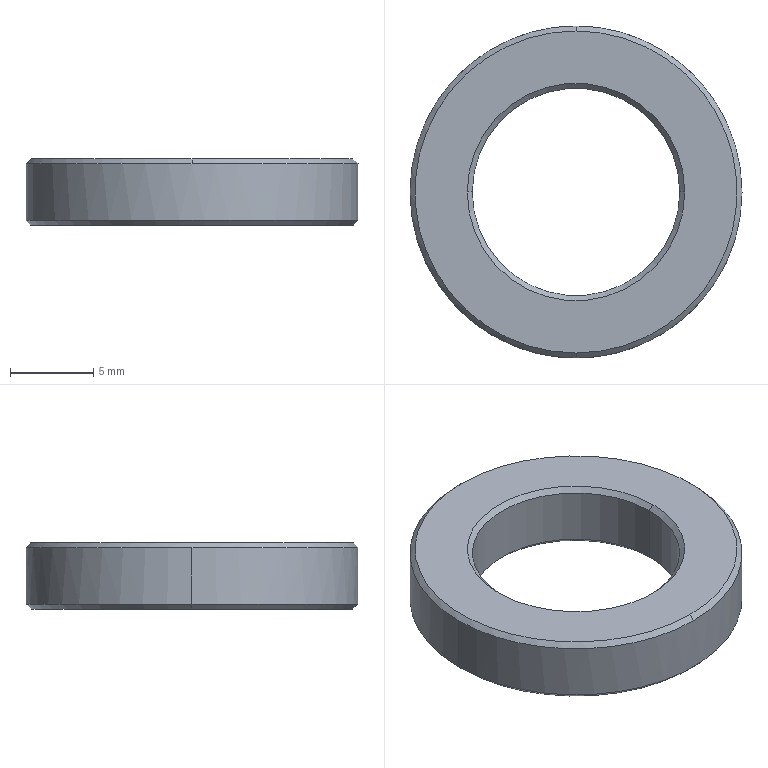Part | STEP file | Bearing locating ring | 1 solid | 14 faces | box 20 x 20 x 4 mm | volume 756.574 mm3 | cone 8 | cylinder 4 | plane 2 | commonest cylinder face diameters 12.5 x2 20 x2
STEP:
#1=CARTESIAN_POINT('',(0.,0.,0.));
#2=DIRECTION('',(0.,0.,1.));
#3=DIRECTION('',(1.,0.,0.));
#4=AXIS2_PLACEMENT_3D('',#1,#2,#3);
#5=CARTESIAN_POINT('',(10.,0.,0.3));
#6=VERTEX_POINT('',#5);
#7=CARTESIAN_POINT('',(-10.,0.,0.3));
#8=VERTEX_POINT('',#7);
#9=CARTESIAN_POINT('',(0.,0.,0.3));
#10=DIRECTION('',(0.,0.,1.));
#11=DIRECTION('',(1.,0.,0.));
#12=AXIS2_PLACEMENT_3D('',#9,#10,#11);
#13=CIRCLE('',#12,10.);
#14=CARTESIAN_POINT('',(0.,0.,0.));
#15=DIRECTION('',(0.,0.,1.));
#16=DIRECTION('',(1.,0.,0.));
#17=AXIS2_PLACEMENT_3D('',#14,#15,#16);
#18=CYLINDRICAL_SURFACE('',#17,10.);
#19=CARTESIAN_POINT('',(0.,0.3));
#20=DIRECTION('',(1.,0.));
#21=VECTOR('',#20,1.);
#22=LINE('',#19,#21);
#23=(GEOMETRIC_REPRESENTATION_CONTEXT(2)PARAMETRIC_REPRESENTATION_CONTEXT()REPRESENTATION_CONTEXT('',''));
#24=DEFINITIONAL_REPRESENTATION('',(#22),#23);
#25=PCURVE('',#18,#24);
#26=CARTESIAN_POINT('',(0.,0.,0.3));
#27=DIRECTION('',(0.,0.,1.));
#28=DIRECTION('',(1.,0.,0.));
#29=AXIS2_PLACEMENT_3D('',#26,#27,#28);
#30=CONICAL_SURFACE('',#29,10.,0.7854);
#31=CARTESIAN_POINT('',(0.,0.));
#32=DIRECTION('',(1.,0.));
#33=VECTOR('',#32,1.);
#34=LINE('',#31,#33);
#35=(GEOMETRIC_REPRESENTATION_CONTEXT(2)PARAMETRIC_REPRESENTATION_CONTEXT()REPRESENTATION_CONTEXT('',''));
#36=DEFINITIONAL_REPRESENTATION('',(#34),#35);
#37=PCURVE('',#30,#36);
#38=SURFACE_CURVE('',#13,(#25,#37),.PCURVE_S1.);
#39=EDGE_CURVE('',#6,#8,#38,.T.);
#40=ORIENTED_EDGE('',*,*,#39,.T.);
#41=CARTESIAN_POINT('',(-10.,0.,3.7));
#42=VERTEX_POINT('',#41);
#43=CARTESIAN_POINT('',(-10.,0.,0.));
#44=DIRECTION('',(0.,0.,1.));
#45=VECTOR('',#44,1.);
#46=LINE('',#43,#45);
#47=CARTESIAN_POINT('',(3.142,0.));
#48=DIRECTION('',(0.,1.));
#49=VECTOR('',#48,1.);
#50=LINE('',#47,#49);
#51=(GEOMETRIC_REPRESENTATION_CONTEXT(2)PARAMETRIC_REPRESENTATION_CONTEXT()REPRESENTATION_CONTEXT('',''));
#52=DEFINITIONAL_REPRESENTATION('',(#50),#51);
#53=PCURVE('',#18,#52);
#54=CARTESIAN_POINT('',(0.,0.,0.));
#55=DIRECTION('',(0.,0.,1.));
#56=DIRECTION('',(1.,0.,0.));
#57=AXIS2_PLACEMENT_3D('',#54,#55,#56);
#58=CYLINDRICAL_SURFACE('',#57,10.);
#59=CARTESIAN_POINT('',(3.142,0.));
#60=DIRECTION('',(0.,1.));
#61=VECTOR('',#60,1.);
#62=LINE('',#59,#61);
#63=(GEOMETRIC_REPRESENTATION_CONTEXT(2)PARAMETRIC_REPRESENTATION_CONTEXT()REPRESENTATION_CONTEXT('',''));
#64=DEFINITIONAL_REPRESENTATION('',(#62),#63);
#65=PCURVE('',#58,#64);
#66=SURFACE_CURVE('',#46,(#53,#65),.PCURVE_S1.);
#67=EDGE_CURVE('',#8,#42,#66,.T.);
#68=ORIENTED_EDGE('',*,*,#67,.T.);
#69=CARTESIAN_POINT('',(0.,10.,3.7));
#70=VERTEX_POINT('',#69);
#71=CARTESIAN_POINT('',(0.,0.,3.7));
#72=DIRECTION('',(0.,0.,-1.));
#73=DIRECTION('',(1.,0.,0.));
#74=AXIS2_PLACEMENT_3D('',#71,#72,#73);
#75=CIRCLE('',#74,10.);
#76=CARTESIAN_POINT('',(6.283,3.7));
#77=DIRECTION('',(-1.,0.));
#78=VECTOR('',#77,1.);
#79=LINE('',#76,#78);
#80=(GEOMETRIC_REPRESENTATION_CONTEXT(2)PARAMETRIC_REPRESENTATION_CONTEXT()REPRESENTATION_CONTEXT('',''));
#81=DEFINITIONAL_REPRESENTATION('',(#79),#80);
#82=PCURVE('',#18,#81);
#83=CARTESIAN_POINT('',(0.,0.,3.7));
#84=DIRECTION('',(0.,0.,-1.));
#85=DIRECTION('',(0.,1.,0.));
#86=AXIS2_PLACEMENT_3D('',#83,#84,#85);
#87=CONICAL_SURFACE('',#86,10.,0.7854);
#88=CARTESIAN_POINT('',(1.571,0.));
#89=DIRECTION('',(1.,0.));
#90=VECTOR('',#89,1.);
#91=LINE('',#88,#90);
#92=(GEOMETRIC_REPRESENTATION_CONTEXT(2)PARAMETRIC_REPRESENTATION_CONTEXT()REPRESENTATION_CONTEXT('',''));
#93=DEFINITIONAL_REPRESENTATION('',(#91),#92);
#94=PCURVE('',#87,#93);
#95=SURFACE_CURVE('',#75,(#82,#94),.PCURVE_S1.);
#96=EDGE_CURVE('',#42,#70,#95,.T.);
#97=ORIENTED_EDGE('',*,*,#96,.T.);
#98=CARTESIAN_POINT('',(10.,0.,3.7));
#99=VERTEX_POINT('',#98);
#100=CARTESIAN_POINT('',(0.,0.,3.7));
#101=DIRECTION('',(0.,0.,-1.));
#102=DIRECTION('',(1.,0.,0.));
#103=AXIS2_PLACEMENT_3D('',#100,#101,#102);
#104=CIRCLE('',#103,10.);
#105=CARTESIAN_POINT('',(6.283,3.7));
#106=DIRECTION('',(-1.,0.));
#107=VECTOR('',#106,1.);
#108=LINE('',#105,#107);
#109=(GEOMETRIC_REPRESENTATION_CONTEXT(2)PARAMETRIC_REPRESENTATION_CONTEXT()REPRESENTATION_CONTEXT('',''));
#110=DEFINITIONAL_REPRESENTATION('',(#108),#109);
#111=PCURVE('',#18,#110);
#112=CARTESIAN_POINT('',(0.,0.,3.7));
#113=DIRECTION('',(0.,0.,-1.));
#114=DIRECTION('',(0.,1.,0.));
#115=AXIS2_PLACEMENT_3D('',#112,#113,#114);
#116=CONICAL_SURFACE('',#115,10.,0.7854);
#117=CARTESIAN_POINT('',(-4.712,0.));
#118=DIRECTION('',(1.,0.));
#119=VECTOR('',#118,1.);
#120=LINE('',#117,#119);
#121=(GEOMETRIC_REPRESENTATION_CONTEXT(2)PARAMETRIC_REPRESENTATION_CONTEXT()REPRESENTATION_CONTEXT('',''));
#122=DEFINITIONAL_REPRESENTATION('',(#120),#121);
#123=PCURVE('',#116,#122);
#124=SURFACE_CURVE('',#104,(#111,#123),.PCURVE_S1.);
#125=EDGE_CURVE('',#70,#99,#124,.T.);
#126=ORIENTED_EDGE('',*,*,#125,.T.);
#127=CARTESIAN_POINT('',(10.,0.,0.));
#128=DIRECTION('',(0.,0.,1.));
#129=VECTOR('',#128,1.);
#130=LINE('',#127,#129);
#131=CARTESIAN_POINT('',(0.,0.));
#132=DIRECTION('',(0.,1.));
#133=VECTOR('',#132,1.);
#134=LINE('',#131,#133);
#135=(GEOMETRIC_REPRESENTATION_CONTEXT(2)PARAMETRIC_REPRESENTATION_CONTEXT()REPRESENTATION_CONTEXT('',''));
#136=DEFINITIONAL_REPRESENTATION('',(#134),#135);
#137=PCURVE('',#18,#136);
#138=CARTESIAN_POINT('',(6.283,0.));
#139=DIRECTION('',(0.,1.));
#140=VECTOR('',#139,1.);
#141=LINE('',#138,#140);
#142=(GEOMETRIC_REPRESENTATION_CONTEXT(2)PARAMETRIC_REPRESENTATION_CONTEXT()REPRESENTATION_CONTEXT('',''));
#143=DEFINITIONAL_REPRESENTATION('',(#141),#142);
#144=PCURVE('',#58,#143);
#145=SURFACE_CURVE('',#130,(#137,#144),.PCURVE_S1.);
#146=EDGE_CURVE('',#6,#99,#145,.T.);
#147=ORIENTED_EDGE('',*,*,#146,.F.);
#148=EDGE_LOOP('',(#40,#68,#97,#126,#147));
#149=FACE_BOUND('',#148,.T.);
#150=ADVANCED_FACE('',(#149),#18,.T.);
#151=CARTESIAN_POINT('',(9.7,0.,0.));
#152=VERTEX_POINT('',#151);
#153=CARTESIAN_POINT('',(-9.7,0.,0.));
#154=VERTEX_POINT('',#153);
#155=CARTESIAN_POINT('',(0.,0.,0.));
#156=DIRECTION('',(0.,0.,1.));
#157=DIRECTION('',(1.,0.,0.));
#158=AXIS2_PLACEMENT_3D('',#155,#156,#157);
#159=CIRCLE('',#158,9.7);
#160=CARTESIAN_POINT('',(0.,-0.3));
#161=DIRECTION('',(1.,0.));
#162=VECTOR('',#161,1.);
#163=LINE('',#160,#162);
#164=(GEOMETRIC_REPRESENTATION_CONTEXT(2)PARAMETRIC_REPRESENTATION_CONTEXT()REPRESENTATION_CONTEXT('',''));
#165=DEFINITIONAL_REPRESENTATION('',(#163),#164);
#166=PCURVE('',#30,#165);
#167=CARTESIAN_POINT('',(0.,0.,0.));
#168=DIRECTION('',(0.,0.,-1.));
#169=DIRECTION('',(-1.,0.,0.));
#170=AXIS2_PLACEMENT_3D('',#167,#168,#169);
#171=PLANE('',#170);
#172=CARTESIAN_POINT('',(-9.7,0.));
#173=CARTESIAN_POINT('',(-9.7,16.801));
#174=CARTESIAN_POINT('',(4.85,8.4));
#175=CARTESIAN_POINT('',(19.4,0.));
#176=CARTESIAN_POINT('',(4.85,-8.4));
#177=CARTESIAN_POINT('',(-9.7,-16.801));
#178=CARTESIAN_POINT('',(-9.7,0.));
#179=(BOUNDED_CURVE()B_SPLINE_CURVE(2,(#172,#173,#174,#175,#176,#177,#178),.UNSPECIFIED.,.T.,.F.)B_SPLINE_CURVE_WITH_KNOTS((1,2,2,2,2,1),(-2.094,0.,2.094,4.189,6.283,8.378),.UNSPECIFIED.)CURVE()GEOMETRIC_REPRESENTATION_ITEM()RATIONAL_B_SPLINE_CURVE((1.,0.5,1.,0.5,1.,0.5,1.))REPRESENTATION_ITEM(''));
#180=(GEOMETRIC_REPRESENTATION_CONTEXT(2)PARAMETRIC_REPRESENTATION_CONTEXT()REPRESENTATION_CONTEXT('',''));
#181=DEFINITIONAL_REPRESENTATION('',(#179),#180);
#182=PCURVE('',#171,#181);
#183=SURFACE_CURVE('',#159,(#166,#182),.PCURVE_S1.);
#184=EDGE_CURVE('',#152,#154,#183,.T.);
#185=ORIENTED_EDGE('',*,*,#184,.T.);
#186=CARTESIAN_POINT('',(-10.,0.,0.3));
#187=DIRECTION('',(-0.7071,0.,0.7071));
#188=VECTOR('',#187,1.);
#189=LINE('',#186,#188);
#190=CARTESIAN_POINT('',(3.142,0.));
#191=DIRECTION('',(0.,1.));
#192=VECTOR('',#191,1.);
#193=LINE('',#190,#192);
#194=(GEOMETRIC_REPRESENTATION_CONTEXT(2)PARAMETRIC_REPRESENTATION_CONTEXT()REPRESENTATION_CONTEXT('',''));
#195=DEFINITIONAL_REPRESENTATION('',(#193),#194);
#196=PCURVE('',#30,#195);
#197=CARTESIAN_POINT('',(0.,0.,0.3));
#198=DIRECTION('',(0.,0.,1.));
#199=DIRECTION('',(1.,0.,0.));
#200=AXIS2_PLACEMENT_3D('',#197,#198,#199);
#201=CONICAL_SURFACE('',#200,10.,0.7854);
#202=CARTESIAN_POINT('',(3.142,0.));
#203=DIRECTION('',(0.,1.));
#204=VECTOR('',#203,1.);
#205=LINE('',#202,#204);
#206=(GEOMETRIC_REPRESENTATION_CONTEXT(2)PARAMETRIC_REPRESENTATION_CONTEXT()REPRESENTATION_CONTEXT('',''));
#207=DEFINITIONAL_REPRESENTATION('',(#205),#206);
#208=PCURVE('',#201,#207);
#209=SURFACE_CURVE('',#189,(#196,#208),.PCURVE_S1.);
#210=EDGE_CURVE('',#154,#8,#209,.T.);
#211=ORIENTED_EDGE('',*,*,#210,.T.);
#212=ORIENTED_EDGE('',*,*,#39,.F.);
#213=CARTESIAN_POINT('',(10.,0.,0.3));
#214=DIRECTION('',(0.7071,0.,0.7071));
#215=VECTOR('',#214,1.);
#216=LINE('',#213,#215);
#217=CARTESIAN_POINT('',(0.,0.));
#218=DIRECTION('',(0.,1.));
#219=VECTOR('',#218,1.);
#220=LINE('',#217,#219);
#221=(GEOMETRIC_REPRESENTATION_CONTEXT(2)PARAMETRIC_REPRESENTATION_CONTEXT()REPRESENTATION_CONTEXT('',''));
#222=DEFINITIONAL_REPRESENTATION('',(#220),#221);
#223=PCURVE('',#30,#222);
#224=CARTESIAN_POINT('',(6.283,0.));
#225=DIRECTION('',(0.,1.));
#226=VECTOR('',#225,1.);
#227=LINE('',#224,#226);
#228=(GEOMETRIC_REPRESENTATION_CONTEXT(2)PARAMETRIC_REPRESENTATION_CONTEXT()REPRESENTATION_CONTEXT('',''));
#229=DEFINITIONAL_REPRESENTATION('',(#227),#228);
#230=PCURVE('',#201,#229);
#231=SURFACE_CURVE('',#216,(#223,#230),.PCURVE_S1.);
#232=EDGE_CURVE('',#152,#6,#231,.T.);
#233=ORIENTED_EDGE('',*,*,#232,.F.);
#234=EDGE_LOOP('',(#185,#211,#212,#233));
#235=FACE_BOUND('',#234,.T.);
#236=ADVANCED_FACE('',(#235),#30,.T.);
#237=CARTESIAN_POINT('',(0.,9.7,4.));
#238=VERTEX_POINT('',#237);
#239=CARTESIAN_POINT('',(0.,-9.7,4.));
#240=VERTEX_POINT('',#239);
#241=CARTESIAN_POINT('',(0.,0.,4.));
#242=DIRECTION('',(0.,0.,-1.));
#243=DIRECTION('',(0.,1.,0.));
#244=AXIS2_PLACEMENT_3D('',#241,#242,#243);
#245=CIRCLE('',#244,9.7);
#246=CARTESIAN_POINT('',(0.,-0.3));
#247=DIRECTION('',(1.,0.));
#248=VECTOR('',#247,1.);
#249=LINE('',#246,#248);
#250=(GEOMETRIC_REPRESENTATION_CONTEXT(2)PARAMETRIC_REPRESENTATION_CONTEXT()REPRESENTATION_CONTEXT('',''));
#251=DEFINITIONAL_REPRESENTATION('',(#249),#250);
#252=PCURVE('',#116,#251);
#253=CARTESIAN_POINT('',(0.,0.,4.));
#254=DIRECTION('',(0.,0.,-1.));
#255=DIRECTION('',(-1.,0.,0.));
#256=AXIS2_PLACEMENT_3D('',#253,#254,#255);
#257=PLANE('',#256);
#258=CARTESIAN_POINT('',(0.,0.));
#259=DIRECTION('',(0.,1.));
#260=AXIS2_PLACEMENT_2D('',#258,#259);
#261=CIRCLE('',#260,9.7);
#262=(GEOMETRIC_REPRESENTATION_CONTEXT(2)PARAMETRIC_REPRESENTATION_CONTEXT()REPRESENTATION_CONTEXT('',''));
#263=DEFINITIONAL_REPRESENTATION('',(#261),#262);
#264=PCURVE('',#257,#263);
#265=SURFACE_CURVE('',#245,(#252,#264),.PCURVE_S1.);
#266=EDGE_CURVE('',#238,#240,#265,.T.);
#267=ORIENTED_EDGE('',*,*,#266,.T.);
#268=CARTESIAN_POINT('',(0.,-10.,3.7));
#269=VERTEX_POINT('',#268);
#270=CARTESIAN_POINT('',(0.,-10.,3.7));
#271=DIRECTION('',(0.,-0.7071,-0.7071));
#272=VECTOR('',#271,1.);
#273=LINE('',#270,#272);
#274=CARTESIAN_POINT('',(3.142,0.));
#275=DIRECTION('',(0.,1.));
#276=VECTOR('',#275,1.);
#277=LINE('',#274,#276);
#278=(GEOMETRIC_REPRESENTATION_CONTEXT(2)PARAMETRIC_REPRESENTATION_CONTEXT()REPRESENTATION_CONTEXT('',''));
#279=DEFINITIONAL_REPRESENTATION('',(#277),#278);
#280=PCURVE('',#116,#279);
#281=CARTESIAN_POINT('',(3.142,0.));
#282=DIRECTION('',(0.,1.));
#283=VECTOR('',#282,1.);
#284=LINE('',#281,#283);
#285=(GEOMETRIC_REPRESENTATION_CONTEXT(2)PARAMETRIC_REPRESENTATION_CONTEXT()REPRESENTATION_CONTEXT('',''));
#286=DEFINITIONAL_REPRESENTATION('',(#284),#285);
#287=PCURVE('',#87,#286);
#288=SURFACE_CURVE('',#273,(#280,#287),.PCURVE_S1.);
#289=EDGE_CURVE('',#240,#269,#288,.T.);
#290=ORIENTED_EDGE('',*,*,#289,.T.);
#291=CARTESIAN_POINT('',(0.,0.,3.7));
#292=DIRECTION('',(0.,0.,-1.));
#293=DIRECTION('',(1.,0.,0.));
#294=AXIS2_PLACEMENT_3D('',#291,#292,#293);
#295=CIRCLE('',#294,10.);
#296=CARTESIAN_POINT('',(1.571,0.));
#297=DIRECTION('',(1.,0.));
#298=VECTOR('',#297,1.);
#299=LINE('',#296,#298);
#300=(GEOMETRIC_REPRESENTATION_CONTEXT(2)PARAMETRIC_REPRESENTATION_CONTEXT()REPRESENTATION_CONTEXT('',''));
#301=DEFINITIONAL_REPRESENTATION('',(#299),#300);
#302=PCURVE('',#116,#301);
#303=CARTESIAN_POINT('',(6.283,3.7));
#304=DIRECTION('',(-1.,0.));
#305=VECTOR('',#304,1.);
#306=LINE('',#303,#305);
#307=(GEOMETRIC_REPRESENTATION_CONTEXT(2)PARAMETRIC_REPRESENTATION_CONTEXT()REPRESENTATION_CONTEXT('',''));
#308=DEFINITIONAL_REPRESENTATION('',(#306),#307);
#309=PCURVE('',#58,#308);
#310=SURFACE_CURVE('',#295,(#302,#309),.PCURVE_S1.);
#311=EDGE_CURVE('',#99,#269,#310,.T.);
#312=ORIENTED_EDGE('',*,*,#311,.F.);
#313=ORIENTED_EDGE('',*,*,#125,.F.);
#314=CARTESIAN_POINT('',(0.,10.,3.7));
#315=DIRECTION('',(0.,0.7071,-0.7071));
#316=VECTOR('',#315,1.);
#317=LINE('',#314,#316);
#318=CARTESIAN_POINT('',(0.,0.));
#319=DIRECTION('',(0.,1.));
#320=VECTOR('',#319,1.);
#321=LINE('',#318,#320);
#322=(GEOMETRIC_REPRESENTATION_CONTEXT(2)PARAMETRIC_REPRESENTATION_CONTEXT()REPRESENTATION_CONTEXT('',''));
#323=DEFINITIONAL_REPRESENTATION('',(#321),#322);
#324=PCURVE('',#116,#323);
#325=CARTESIAN_POINT('',(6.283,0.));
#326=DIRECTION('',(0.,1.));
#327=VECTOR('',#326,1.);
#328=LINE('',#325,#327);
#329=(GEOMETRIC_REPRESENTATION_CONTEXT(2)PARAMETRIC_REPRESENTATION_CONTEXT()REPRESENTATION_CONTEXT('',''));
#330=DEFINITIONAL_REPRESENTATION('',(#328),#329);
#331=PCURVE('',#87,#330);
#332=SURFACE_CURVE('',#317,(#324,#331),.PCURVE_S1.);
#333=EDGE_CURVE('',#238,#70,#332,.T.);
#334=ORIENTED_EDGE('',*,*,#333,.F.);
#335=EDGE_LOOP('',(#267,#290,#312,#313,#334));
#336=FACE_BOUND('',#335,.T.);
#337=ADVANCED_FACE('',(#336),#116,.T.);
#338=CARTESIAN_POINT('',(-6.25,0.,0.3));
#339=VERTEX_POINT('',#338);
#340=CARTESIAN_POINT('',(-6.55,0.,0.));
#341=VERTEX_POINT('',#340);
#342=CARTESIAN_POINT('',(-6.55,0.,0.));
#343=DIRECTION('',(-0.7071,0.,-0.7071));
#344=VECTOR('',#343,1.);
#345=LINE('',#342,#344);
#346=CARTESIAN_POINT('',(0.,0.,0.));
#347=DIRECTION('',(0.,0.,-1.));
#348=DIRECTION('',(-1.,0.,0.));
#349=AXIS2_PLACEMENT_3D('',#346,#347,#348);
#350=CONICAL_SURFACE('',#349,6.55,0.7854);
#351=CARTESIAN_POINT('',(6.283,0.));
#352=DIRECTION('',(0.,1.));
#353=VECTOR('',#352,1.);
#354=LINE('',#351,#353);
#355=(GEOMETRIC_REPRESENTATION_CONTEXT(2)PARAMETRIC_REPRESENTATION_CONTEXT()REPRESENTATION_CONTEXT('',''));
#356=DEFINITIONAL_REPRESENTATION('',(#354),#355);
#357=PCURVE('',#350,#356);
#358=CARTESIAN_POINT('',(0.,0.,0.));
#359=DIRECTION('',(0.,0.,-1.));
#360=DIRECTION('',(-1.,0.,0.));
#361=AXIS2_PLACEMENT_3D('',#358,#359,#360);
#362=CONICAL_SURFACE('',#361,6.55,0.7854);
#363=CARTESIAN_POINT('',(0.,0.));
#364=DIRECTION('',(0.,1.));
#365=VECTOR('',#364,1.);
#366=LINE('',#363,#365);
#367=(GEOMETRIC_REPRESENTATION_CONTEXT(2)PARAMETRIC_REPRESENTATION_CONTEXT()REPRESENTATION_CONTEXT('',''));
#368=DEFINITIONAL_REPRESENTATION('',(#366),#367);
#369=PCURVE('',#362,#368);
#370=SURFACE_CURVE('',#345,(#357,#369),.PCURVE_S1.);
#371=EDGE_CURVE('',#339,#341,#370,.T.);
#372=ORIENTED_EDGE('',*,*,#371,.T.);
#373=CARTESIAN_POINT('',(6.55,0.,0.));
#374=VERTEX_POINT('',#373);
#375=CARTESIAN_POINT('',(0.,0.,0.));
#376=DIRECTION('',(0.,0.,1.));
#377=DIRECTION('',(-1.,0.,0.));
#378=AXIS2_PLACEMENT_3D('',#375,#376,#377);
#379=CIRCLE('',#378,6.55);
#380=CARTESIAN_POINT('',(6.283,0.));
#381=DIRECTION('',(-1.,0.));
#382=VECTOR('',#381,1.);
#383=LINE('',#380,#382);
#384=(GEOMETRIC_REPRESENTATION_CONTEXT(2)PARAMETRIC_REPRESENTATION_CONTEXT()REPRESENTATION_CONTEXT('',''));
#385=DEFINITIONAL_REPRESENTATION('',(#383),#384);
#386=PCURVE('',#350,#385);
#387=CARTESIAN_POINT('',(6.55,0.));
#388=CARTESIAN_POINT('',(6.55,-11.345));
#389=CARTESIAN_POINT('',(-3.275,-5.672));
#390=CARTESIAN_POINT('',(-13.1,0.));
#391=CARTESIAN_POINT('',(-3.275,5.672));
#392=CARTESIAN_POINT('',(6.55,11.345));
#393=CARTESIAN_POINT('',(6.55,0.));
#394=(BOUNDED_CURVE()B_SPLINE_CURVE(2,(#387,#388,#389,#390,#391,#392,#393),.UNSPECIFIED.,.T.,.F.)B_SPLINE_CURVE_WITH_KNOTS((1,2,2,2,2,1),(-2.094,0.,2.094,4.189,6.283,8.378),.UNSPECIFIED.)CURVE()GEOMETRIC_REPRESENTATION_ITEM()RATIONAL_B_SPLINE_CURVE((1.,0.5,1.,0.5,1.,0.5,1.))REPRESENTATION_ITEM(''));
#395=(GEOMETRIC_REPRESENTATION_CONTEXT(2)PARAMETRIC_REPRESENTATION_CONTEXT()REPRESENTATION_CONTEXT('',''));
#396=DEFINITIONAL_REPRESENTATION('',(#394),#395);
#397=PCURVE('',#171,#396);
#398=SURFACE_CURVE('',#379,(#386,#397),.PCURVE_S1.);
#399=EDGE_CURVE('',#341,#374,#398,.T.);
#400=ORIENTED_EDGE('',*,*,#399,.T.);
#401=CARTESIAN_POINT('',(6.25,0.,0.3));
#402=VERTEX_POINT('',#401);
#403=CARTESIAN_POINT('',(6.55,0.,0.));
#404=DIRECTION('',(0.7071,0.,-0.7071));
#405=VECTOR('',#404,1.);
#406=LINE('',#403,#405);
#407=CARTESIAN_POINT('',(3.142,0.));
#408=DIRECTION('',(0.,1.));
#409=VECTOR('',#408,1.);
#410=LINE('',#407,#409);
#411=(GEOMETRIC_REPRESENTATION_CONTEXT(2)PARAMETRIC_REPRESENTATION_CONTEXT()REPRESENTATION_CONTEXT('',''));
#412=DEFINITIONAL_REPRESENTATION('',(#410),#411);
#413=PCURVE('',#350,#412);
#414=CARTESIAN_POINT('',(3.142,0.));
#415=DIRECTION('',(0.,1.));
#416=VECTOR('',#415,1.);
#417=LINE('',#414,#416);
#418=(GEOMETRIC_REPRESENTATION_CONTEXT(2)PARAMETRIC_REPRESENTATION_CONTEXT()REPRESENTATION_CONTEXT('',''));
#419=DEFINITIONAL_REPRESENTATION('',(#417),#418);
#420=PCURVE('',#362,#419);
#421=SURFACE_CURVE('',#406,(#413,#420),.PCURVE_S1.);
#422=EDGE_CURVE('',#402,#374,#421,.T.);
#423=ORIENTED_EDGE('',*,*,#422,.F.);
#424=CARTESIAN_POINT('',(0.,0.,0.3));
#425=DIRECTION('',(0.,0.,-1.));
#426=DIRECTION('',(-1.,0.,0.));
#427=AXIS2_PLACEMENT_3D('',#424,#425,#426);
#428=CIRCLE('',#427,6.25);
#429=CARTESIAN_POINT('',(0.,-0.3));
#430=DIRECTION('',(1.,0.));
#431=VECTOR('',#430,1.);
#432=LINE('',#429,#431);
#433=(GEOMETRIC_REPRESENTATION_CONTEXT(2)PARAMETRIC_REPRESENTATION_CONTEXT()REPRESENTATION_CONTEXT('',''));
#434=DEFINITIONAL_REPRESENTATION('',(#432),#433);
#435=PCURVE('',#350,#434);
#436=CARTESIAN_POINT('',(0.,0.,0.));
#437=DIRECTION('',(0.,0.,1.));
#438=DIRECTION('',(1.,0.,0.));
#439=AXIS2_PLACEMENT_3D('',#436,#437,#438);
#440=CYLINDRICAL_SURFACE('',#439,6.25);
#441=CARTESIAN_POINT('',(9.425,0.3));
#442=DIRECTION('',(-1.,0.));
#443=VECTOR('',#442,1.);
#444=LINE('',#441,#443);
#445=(GEOMETRIC_REPRESENTATION_CONTEXT(2)PARAMETRIC_REPRESENTATION_CONTEXT()REPRESENTATION_CONTEXT('',''));
#446=DEFINITIONAL_REPRESENTATION('',(#444),#445);
#447=PCURVE('',#440,#446);
#448=SURFACE_CURVE('',#428,(#435,#447),.PCURVE_S1.);
#449=EDGE_CURVE('',#402,#339,#448,.T.);
#450=ORIENTED_EDGE('',*,*,#449,.T.);
#451=EDGE_LOOP('',(#372,#400,#423,#450));
#452=FACE_BOUND('',#451,.F.);
#453=ADVANCED_FACE('',(#452),#350,.F.);
#454=CARTESIAN_POINT('',(6.25,0.,3.7));
#455=VERTEX_POINT('',#454);
#456=CARTESIAN_POINT('',(6.55,0.,4.));
#457=VERTEX_POINT('',#456);
#458=CARTESIAN_POINT('',(6.55,0.,4.));
#459=DIRECTION('',(0.7071,0.,0.7071));
#460=VECTOR('',#459,1.);
#461=LINE('',#458,#460);
#462=CARTESIAN_POINT('',(0.,0.,4.));
#463=DIRECTION('',(0.,0.,1.));
#464=DIRECTION('',(1.,0.,0.));
#465=AXIS2_PLACEMENT_3D('',#462,#463,#464);
#466=CONICAL_SURFACE('',#465,6.55,0.7854);
#467=CARTESIAN_POINT('',(6.283,0.));
#468=DIRECTION('',(0.,1.));
#469=VECTOR('',#468,1.);
#470=LINE('',#467,#469);
#471=(GEOMETRIC_REPRESENTATION_CONTEXT(2)PARAMETRIC_REPRESENTATION_CONTEXT()REPRESENTATION_CONTEXT('',''));
#472=DEFINITIONAL_REPRESENTATION('',(#470),#471);
#473=PCURVE('',#466,#472);
#474=CARTESIAN_POINT('',(0.,0.,4.));
#475=DIRECTION('',(0.,0.,1.));
#476=DIRECTION('',(1.,0.,0.));
#477=AXIS2_PLACEMENT_3D('',#474,#475,#476);
#478=CONICAL_SURFACE('',#477,6.55,0.7854);
#479=CARTESIAN_POINT('',(0.,0.));
#480=DIRECTION('',(0.,1.));
#481=VECTOR('',#480,1.);
#482=LINE('',#479,#481);
#483=(GEOMETRIC_REPRESENTATION_CONTEXT(2)PARAMETRIC_REPRESENTATION_CONTEXT()REPRESENTATION_CONTEXT('',''));
#484=DEFINITIONAL_REPRESENTATION('',(#482),#483);
#485=PCURVE('',#478,#484);
#486=SURFACE_CURVE('',#461,(#473,#485),.PCURVE_S1.);
#487=EDGE_CURVE('',#455,#457,#486,.T.);
#488=ORIENTED_EDGE('',*,*,#487,.T.);
#489=CARTESIAN_POINT('',(-6.55,0.,4.));
#490=VERTEX_POINT('',#489);
#491=CARTESIAN_POINT('',(0.,0.,4.));
#492=DIRECTION('',(0.,0.,1.));
#493=DIRECTION('',(1.,0.,0.));
#494=AXIS2_PLACEMENT_3D('',#491,#492,#493);
#495=CIRCLE('',#494,6.55);
#496=CARTESIAN_POINT('',(0.,0.));
#497=DIRECTION('',(1.,0.));
#498=VECTOR('',#497,1.);
#499=LINE('',#496,#498);
#500=(GEOMETRIC_REPRESENTATION_CONTEXT(2)PARAMETRIC_REPRESENTATION_CONTEXT()REPRESENTATION_CONTEXT('',''));
#501=DEFINITIONAL_REPRESENTATION('',(#499),#500);
#502=PCURVE('',#466,#501);
#503=CARTESIAN_POINT('',(-6.55,0.));
#504=CARTESIAN_POINT('',(-6.55,11.345));
#505=CARTESIAN_POINT('',(3.275,5.672));
#506=CARTESIAN_POINT('',(13.1,0.));
#507=CARTESIAN_POINT('',(3.275,-5.672));
#508=CARTESIAN_POINT('',(-6.55,-11.345));
#509=CARTESIAN_POINT('',(-6.55,0.));
#510=(BOUNDED_CURVE()B_SPLINE_CURVE(2,(#503,#504,#505,#506,#507,#508,#509),.UNSPECIFIED.,.T.,.F.)B_SPLINE_CURVE_WITH_KNOTS((1,2,2,2,2,1),(-2.094,0.,2.094,4.189,6.283,8.378),.UNSPECIFIED.)CURVE()GEOMETRIC_REPRESENTATION_ITEM()RATIONAL_B_SPLINE_CURVE((1.,0.5,1.,0.5,1.,0.5,1.))REPRESENTATION_ITEM(''));
#511=(GEOMETRIC_REPRESENTATION_CONTEXT(2)PARAMETRIC_REPRESENTATION_CONTEXT()REPRESENTATION_CONTEXT('',''));
#512=DEFINITIONAL_REPRESENTATION('',(#510),#511);
#513=PCURVE('',#257,#512);
#514=SURFACE_CURVE('',#495,(#502,#513),.PCURVE_S1.);
#515=EDGE_CURVE('',#490,#457,#514,.T.);
#516=ORIENTED_EDGE('',*,*,#515,.F.);
#517=CARTESIAN_POINT('',(-6.25,0.,3.7));
#518=VERTEX_POINT('',#517);
#519=CARTESIAN_POINT('',(-6.55,0.,4.));
#520=DIRECTION('',(-0.7071,0.,0.7071));
#521=VECTOR('',#520,1.);
#522=LINE('',#519,#521);
#523=CARTESIAN_POINT('',(3.142,0.));
#524=DIRECTION('',(0.,1.));
#525=VECTOR('',#524,1.);
#526=LINE('',#523,#525);
#527=(GEOMETRIC_REPRESENTATION_CONTEXT(2)PARAMETRIC_REPRESENTATION_CONTEXT()REPRESENTATION_CONTEXT('',''));
#528=DEFINITIONAL_REPRESENTATION('',(#526),#527);
#529=PCURVE('',#466,#528);
#530=CARTESIAN_POINT('',(3.142,0.));
#531=DIRECTION('',(0.,1.));
#532=VECTOR('',#531,1.);
#533=LINE('',#530,#532);
#534=(GEOMETRIC_REPRESENTATION_CONTEXT(2)PARAMETRIC_REPRESENTATION_CONTEXT()REPRESENTATION_CONTEXT('',''));
#535=DEFINITIONAL_REPRESENTATION('',(#533),#534);
#536=PCURVE('',#478,#535);
#537=SURFACE_CURVE('',#522,(#529,#536),.PCURVE_S1.);
#538=EDGE_CURVE('',#518,#490,#537,.T.);
#539=ORIENTED_EDGE('',*,*,#538,.F.);
#540=CARTESIAN_POINT('',(0.,0.,3.7));
#541=DIRECTION('',(0.,0.,1.));
#542=DIRECTION('',(-1.,0.,0.));
#543=AXIS2_PLACEMENT_3D('',#540,#541,#542);
#544=CIRCLE('',#543,6.25);
#545=CARTESIAN_POINT('',(3.142,-0.3));
#546=DIRECTION('',(1.,0.));
#547=VECTOR('',#546,1.);
#548=LINE('',#545,#547);
#549=(GEOMETRIC_REPRESENTATION_CONTEXT(2)PARAMETRIC_REPRESENTATION_CONTEXT()REPRESENTATION_CONTEXT('',''));
#550=DEFINITIONAL_REPRESENTATION('',(#548),#549);
#551=PCURVE('',#466,#550);
#552=CARTESIAN_POINT('',(3.142,3.7));
#553=DIRECTION('',(1.,0.));
#554=VECTOR('',#553,1.);
#555=LINE('',#552,#554);
#556=(GEOMETRIC_REPRESENTATION_CONTEXT(2)PARAMETRIC_REPRESENTATION_CONTEXT()REPRESENTATION_CONTEXT('',''));
#557=DEFINITIONAL_REPRESENTATION('',(#555),#556);
#558=PCURVE('',#440,#557);
#559=SURFACE_CURVE('',#544,(#551,#558),.PCURVE_S1.);
#560=EDGE_CURVE('',#518,#455,#559,.T.);
#561=ORIENTED_EDGE('',*,*,#560,.T.);
#562=EDGE_LOOP('',(#488,#516,#539,#561));
#563=FACE_BOUND('',#562,.F.);
#564=ADVANCED_FACE('',(#563),#466,.F.);
#565=CARTESIAN_POINT('',(6.25,0.,0.));
#566=DIRECTION('',(0.,0.,1.));
#567=VECTOR('',#566,1.);
#568=LINE('',#565,#567);
#569=CARTESIAN_POINT('',(6.283,0.));
#570=DIRECTION('',(0.,1.));
#571=VECTOR('',#570,1.);
#572=LINE('',#569,#571);
#573=(GEOMETRIC_REPRESENTATION_CONTEXT(2)PARAMETRIC_REPRESENTATION_CONTEXT()REPRESENTATION_CONTEXT('',''));
#574=DEFINITIONAL_REPRESENTATION('',(#572),#573);
#575=PCURVE('',#440,#574);
#576=CARTESIAN_POINT('',(0.,0.,0.));
#577=DIRECTION('',(0.,0.,1.));
#578=DIRECTION('',(1.,0.,0.));
#579=AXIS2_PLACEMENT_3D('',#576,#577,#578);
#580=CYLINDRICAL_SURFACE('',#579,6.25);
#581=CARTESIAN_POINT('',(0.,0.));
#582=DIRECTION('',(0.,1.));
#583=VECTOR('',#582,1.);
#584=LINE('',#581,#583);
#585=(GEOMETRIC_REPRESENTATION_CONTEXT(2)PARAMETRIC_REPRESENTATION_CONTEXT()REPRESENTATION_CONTEXT('',''));
#586=DEFINITIONAL_REPRESENTATION('',(#584),#585);
#587=PCURVE('',#580,#586);
#588=SURFACE_CURVE('',#568,(#575,#587),.PCURVE_S1.);
#589=EDGE_CURVE('',#402,#455,#588,.T.);
#590=ORIENTED_EDGE('',*,*,#589,.T.);
#591=ORIENTED_EDGE('',*,*,#560,.F.);
#592=CARTESIAN_POINT('',(-6.25,0.,0.));
#593=DIRECTION('',(0.,0.,1.));
#594=VECTOR('',#593,1.);
#595=LINE('',#592,#594);
#596=CARTESIAN_POINT('',(3.142,0.));
#597=DIRECTION('',(0.,1.));
#598=VECTOR('',#597,1.);
#599=LINE('',#596,#598);
#600=(GEOMETRIC_REPRESENTATION_CONTEXT(2)PARAMETRIC_REPRESENTATION_CONTEXT()REPRESENTATION_CONTEXT('',''));
#601=DEFINITIONAL_REPRESENTATION('',(#599),#600);
#602=PCURVE('',#440,#601);
#603=CARTESIAN_POINT('',(3.142,0.));
#604=DIRECTION('',(0.,1.));
#605=VECTOR('',#604,1.);
#606=LINE('',#603,#605);
#607=(GEOMETRIC_REPRESENTATION_CONTEXT(2)PARAMETRIC_REPRESENTATION_CONTEXT()REPRESENTATION_CONTEXT('',''));
#608=DEFINITIONAL_REPRESENTATION('',(#606),#607);
#609=PCURVE('',#580,#608);
#610=SURFACE_CURVE('',#595,(#602,#609),.PCURVE_S1.);
#611=EDGE_CURVE('',#339,#518,#610,.T.);
#612=ORIENTED_EDGE('',*,*,#611,.F.);
#613=ORIENTED_EDGE('',*,*,#449,.F.);
#614=EDGE_LOOP('',(#590,#591,#612,#613));
#615=FACE_BOUND('',#614,.F.);
#616=ADVANCED_FACE('',(#615),#440,.F.);
#617=ORIENTED_EDGE('',*,*,#67,.F.);
#618=CARTESIAN_POINT('',(0.,0.,0.3));
#619=DIRECTION('',(0.,0.,1.));
#620=DIRECTION('',(1.,0.,0.));
#621=AXIS2_PLACEMENT_3D('',#618,#619,#620);
#622=CIRCLE('',#621,10.);
#623=CARTESIAN_POINT('',(0.,0.3));
#624=DIRECTION('',(1.,0.));
#625=VECTOR('',#624,1.);
#626=LINE('',#623,#625);
#627=(GEOMETRIC_REPRESENTATION_CONTEXT(2)PARAMETRIC_REPRESENTATION_CONTEXT()REPRESENTATION_CONTEXT('',''));
#628=DEFINITIONAL_REPRESENTATION('',(#626),#627);
#629=PCURVE('',#58,#628);
#630=CARTESIAN_POINT('',(0.,0.));
#631=DIRECTION('',(1.,0.));
#632=VECTOR('',#631,1.);
#633=LINE('',#630,#632);
#634=(GEOMETRIC_REPRESENTATION_CONTEXT(2)PARAMETRIC_REPRESENTATION_CONTEXT()REPRESENTATION_CONTEXT('',''));
#635=DEFINITIONAL_REPRESENTATION('',(#633),#634);
#636=PCURVE('',#201,#635);
#637=SURFACE_CURVE('',#622,(#629,#636),.PCURVE_S1.);
#638=EDGE_CURVE('',#8,#6,#637,.T.);
#639=ORIENTED_EDGE('',*,*,#638,.T.);
#640=ORIENTED_EDGE('',*,*,#146,.T.);
#641=ORIENTED_EDGE('',*,*,#311,.T.);
#642=CARTESIAN_POINT('',(0.,0.,3.7));
#643=DIRECTION('',(0.,0.,-1.));
#644=DIRECTION('',(1.,0.,0.));
#645=AXIS2_PLACEMENT_3D('',#642,#643,#644);
#646=CIRCLE('',#645,10.);
#647=CARTESIAN_POINT('',(6.283,3.7));
#648=DIRECTION('',(-1.,0.));
#649=VECTOR('',#648,1.);
#650=LINE('',#647,#649);
#651=(GEOMETRIC_REPRESENTATION_CONTEXT(2)PARAMETRIC_REPRESENTATION_CONTEXT()REPRESENTATION_CONTEXT('',''));
#652=DEFINITIONAL_REPRESENTATION('',(#650),#651);
#653=PCURVE('',#58,#652);
#654=CARTESIAN_POINT('',(1.571,0.));
#655=DIRECTION('',(1.,0.));
#656=VECTOR('',#655,1.);
#657=LINE('',#654,#656);
#658=(GEOMETRIC_REPRESENTATION_CONTEXT(2)PARAMETRIC_REPRESENTATION_CONTEXT()REPRESENTATION_CONTEXT('',''));
#659=DEFINITIONAL_REPRESENTATION('',(#657),#658);
#660=PCURVE('',#87,#659);
#661=SURFACE_CURVE('',#646,(#653,#660),.PCURVE_S1.);
#662=EDGE_CURVE('',#269,#42,#661,.T.);
#663=ORIENTED_EDGE('',*,*,#662,.T.);
#664=EDGE_LOOP('',(#617,#639,#640,#641,#663));
#665=FACE_BOUND('',#664,.T.);
#666=ADVANCED_FACE('',(#665),#58,.T.);
#667=ORIENTED_EDGE('',*,*,#210,.F.);
#668=CARTESIAN_POINT('',(0.,0.,0.));
#669=DIRECTION('',(0.,0.,1.));
#670=DIRECTION('',(1.,0.,0.));
#671=AXIS2_PLACEMENT_3D('',#668,#669,#670);
#672=CIRCLE('',#671,9.7);
#673=CARTESIAN_POINT('',(0.,-0.3));
#674=DIRECTION('',(1.,0.));
#675=VECTOR('',#674,1.);
#676=LINE('',#673,#675);
#677=(GEOMETRIC_REPRESENTATION_CONTEXT(2)PARAMETRIC_REPRESENTATION_CONTEXT()REPRESENTATION_CONTEXT('',''));
#678=DEFINITIONAL_REPRESENTATION('',(#676),#677);
#679=PCURVE('',#201,#678);
#680=CARTESIAN_POINT('',(-9.7,0.));
#681=CARTESIAN_POINT('',(-9.7,16.801));
#682=CARTESIAN_POINT('',(4.85,8.4));
#683=CARTESIAN_POINT('',(19.4,0.));
#684=CARTESIAN_POINT('',(4.85,-8.4));
#685=CARTESIAN_POINT('',(-9.7,-16.801));
#686=CARTESIAN_POINT('',(-9.7,0.));
#687=(BOUNDED_CURVE()B_SPLINE_CURVE(2,(#680,#681,#682,#683,#684,#685,#686),.UNSPECIFIED.,.T.,.F.)B_SPLINE_CURVE_WITH_KNOTS((1,2,2,2,2,1),(-2.094,0.,2.094,4.189,6.283,8.378),.UNSPECIFIED.)CURVE()GEOMETRIC_REPRESENTATION_ITEM()RATIONAL_B_SPLINE_CURVE((1.,0.5,1.,0.5,1.,0.5,1.))REPRESENTATION_ITEM(''));
#688=(GEOMETRIC_REPRESENTATION_CONTEXT(2)PARAMETRIC_REPRESENTATION_CONTEXT()REPRESENTATION_CONTEXT('',''));
#689=DEFINITIONAL_REPRESENTATION('',(#687),#688);
#690=PCURVE('',#171,#689);
#691=SURFACE_CURVE('',#672,(#679,#690),.PCURVE_S1.);
#692=EDGE_CURVE('',#154,#152,#691,.T.);
#693=ORIENTED_EDGE('',*,*,#692,.T.);
#694=ORIENTED_EDGE('',*,*,#232,.T.);
#695=ORIENTED_EDGE('',*,*,#638,.F.);
#696=EDGE_LOOP('',(#667,#693,#694,#695));
#697=FACE_BOUND('',#696,.T.);
#698=ADVANCED_FACE('',(#697),#201,.T.);
#699=ORIENTED_EDGE('',*,*,#289,.F.);
#700=CARTESIAN_POINT('',(0.,0.,4.));
#701=DIRECTION('',(0.,0.,-1.));
#702=DIRECTION('',(0.,1.,0.));
#703=AXIS2_PLACEMENT_3D('',#700,#701,#702);
#704=CIRCLE('',#703,9.7);
#705=CARTESIAN_POINT('',(0.,-0.3));
#706=DIRECTION('',(1.,0.));
#707=VECTOR('',#706,1.);
#708=LINE('',#705,#707);
#709=(GEOMETRIC_REPRESENTATION_CONTEXT(2)PARAMETRIC_REPRESENTATION_CONTEXT()REPRESENTATION_CONTEXT('',''));
#710=DEFINITIONAL_REPRESENTATION('',(#708),#709);
#711=PCURVE('',#87,#710);
#712=CARTESIAN_POINT('',(0.,0.));
#713=DIRECTION('',(0.,1.));
#714=AXIS2_PLACEMENT_2D('',#712,#713);
#715=CIRCLE('',#714,9.7);
#716=(GEOMETRIC_REPRESENTATION_CONTEXT(2)PARAMETRIC_REPRESENTATION_CONTEXT()REPRESENTATION_CONTEXT('',''));
#717=DEFINITIONAL_REPRESENTATION('',(#715),#716);
#718=PCURVE('',#257,#717);
#719=SURFACE_CURVE('',#704,(#711,#718),.PCURVE_S1.);
#720=EDGE_CURVE('',#240,#238,#719,.T.);
#721=ORIENTED_EDGE('',*,*,#720,.T.);
#722=ORIENTED_EDGE('',*,*,#333,.T.);
#723=ORIENTED_EDGE('',*,*,#96,.F.);
#724=ORIENTED_EDGE('',*,*,#662,.F.);
#725=EDGE_LOOP('',(#699,#721,#722,#723,#724));
#726=FACE_BOUND('',#725,.T.);
#727=ADVANCED_FACE('',(#726),#87,.T.);
#728=ORIENTED_EDGE('',*,*,#399,.T.);
#729=CARTESIAN_POINT('',(0.,0.,0.));
#730=DIRECTION('',(0.,0.,1.));
#731=DIRECTION('',(-1.,0.,0.));
#732=AXIS2_PLACEMENT_3D('',#729,#730,#731);
#733=CIRCLE('',#732,6.55);
#734=CARTESIAN_POINT('',(6.55,0.));
#735=CARTESIAN_POINT('',(6.55,-11.345));
#736=CARTESIAN_POINT('',(-3.275,-5.672));
#737=CARTESIAN_POINT('',(-13.1,0.));
#738=CARTESIAN_POINT('',(-3.275,5.672));
#739=CARTESIAN_POINT('',(6.55,11.345));
#740=CARTESIAN_POINT('',(6.55,0.));
#741=(BOUNDED_CURVE()B_SPLINE_CURVE(2,(#734,#735,#736,#737,#738,#739,#740),.UNSPECIFIED.,.T.,.F.)B_SPLINE_CURVE_WITH_KNOTS((1,2,2,2,2,1),(-2.094,0.,2.094,4.189,6.283,8.378),.UNSPECIFIED.)CURVE()GEOMETRIC_REPRESENTATION_ITEM()RATIONAL_B_SPLINE_CURVE((1.,0.5,1.,0.5,1.,0.5,1.))REPRESENTATION_ITEM(''));
#742=(GEOMETRIC_REPRESENTATION_CONTEXT(2)PARAMETRIC_REPRESENTATION_CONTEXT()REPRESENTATION_CONTEXT('',''));
#743=DEFINITIONAL_REPRESENTATION('',(#741),#742);
#744=PCURVE('',#171,#743);
#745=CARTESIAN_POINT('',(6.283,0.));
#746=DIRECTION('',(-1.,0.));
#747=VECTOR('',#746,1.);
#748=LINE('',#745,#747);
#749=(GEOMETRIC_REPRESENTATION_CONTEXT(2)PARAMETRIC_REPRESENTATION_CONTEXT()REPRESENTATION_CONTEXT('',''));
#750=DEFINITIONAL_REPRESENTATION('',(#748),#749);
#751=PCURVE('',#362,#750);
#752=SURFACE_CURVE('',#733,(#744,#751),.PCURVE_S1.);
#753=EDGE_CURVE('',#374,#341,#752,.T.);
#754=ORIENTED_EDGE('',*,*,#753,.T.);
#755=EDGE_LOOP('',(#728,#754));
#756=FACE_BOUND('',#755,.T.);
#757=ORIENTED_EDGE('',*,*,#184,.F.);
#758=ORIENTED_EDGE('',*,*,#692,.F.);
#759=EDGE_LOOP('',(#757,#758));
#760=FACE_BOUND('',#759,.T.);
#761=ADVANCED_FACE('',(#756,#760),#171,.T.);
#762=CARTESIAN_POINT('',(0.,0.,4.));
#763=DIRECTION('',(0.,0.,1.));
#764=DIRECTION('',(1.,0.,0.));
#765=AXIS2_PLACEMENT_3D('',#762,#763,#764);
#766=CIRCLE('',#765,6.55);
#767=CARTESIAN_POINT('',(-6.55,0.));
#768=CARTESIAN_POINT('',(-6.55,11.345));
#769=CARTESIAN_POINT('',(3.275,5.672));
#770=CARTESIAN_POINT('',(13.1,0.));
#771=CARTESIAN_POINT('',(3.275,-5.672));
#772=CARTESIAN_POINT('',(-6.55,-11.345));
#773=CARTESIAN_POINT('',(-6.55,0.));
#774=(BOUNDED_CURVE()B_SPLINE_CURVE(2,(#767,#768,#769,#770,#771,#772,#773),.UNSPECIFIED.,.T.,.F.)B_SPLINE_CURVE_WITH_KNOTS((1,2,2,2,2,1),(-2.094,0.,2.094,4.189,6.283,8.378),.UNSPECIFIED.)CURVE()GEOMETRIC_REPRESENTATION_ITEM()RATIONAL_B_SPLINE_CURVE((1.,0.5,1.,0.5,1.,0.5,1.))REPRESENTATION_ITEM(''));
#775=(GEOMETRIC_REPRESENTATION_CONTEXT(2)PARAMETRIC_REPRESENTATION_CONTEXT()REPRESENTATION_CONTEXT('',''));
#776=DEFINITIONAL_REPRESENTATION('',(#774),#775);
#777=PCURVE('',#257,#776);
#778=CARTESIAN_POINT('',(0.,0.));
#779=DIRECTION('',(1.,0.));
#780=VECTOR('',#779,1.);
#781=LINE('',#778,#780);
#782=(GEOMETRIC_REPRESENTATION_CONTEXT(2)PARAMETRIC_REPRESENTATION_CONTEXT()REPRESENTATION_CONTEXT('',''));
#783=DEFINITIONAL_REPRESENTATION('',(#781),#782);
#784=PCURVE('',#478,#783);
#785=SURFACE_CURVE('',#766,(#777,#784),.PCURVE_S1.);
#786=EDGE_CURVE('',#457,#490,#785,.T.);
#787=ORIENTED_EDGE('',*,*,#786,.F.);
#788=ORIENTED_EDGE('',*,*,#515,.F.);
#789=EDGE_LOOP('',(#787,#788));
#790=FACE_BOUND('',#789,.T.);
#791=ORIENTED_EDGE('',*,*,#266,.F.);
#792=ORIENTED_EDGE('',*,*,#720,.F.);
#793=EDGE_LOOP('',(#791,#792));
#794=FACE_BOUND('',#793,.T.);
#795=ADVANCED_FACE('',(#790,#794),#257,.F.);
#796=ORIENTED_EDGE('',*,*,#753,.T.);
#797=ORIENTED_EDGE('',*,*,#371,.F.);
#798=CARTESIAN_POINT('',(0.,0.,0.3));
#799=DIRECTION('',(0.,0.,-1.));
#800=DIRECTION('',(-1.,0.,0.));
#801=AXIS2_PLACEMENT_3D('',#798,#799,#800);
#802=CIRCLE('',#801,6.25);
#803=CARTESIAN_POINT('',(0.,-0.3));
#804=DIRECTION('',(1.,0.));
#805=VECTOR('',#804,1.);
#806=LINE('',#803,#805);
#807=(GEOMETRIC_REPRESENTATION_CONTEXT(2)PARAMETRIC_REPRESENTATION_CONTEXT()REPRESENTATION_CONTEXT('',''));
#808=DEFINITIONAL_REPRESENTATION('',(#806),#807);
#809=PCURVE('',#362,#808);
#810=CARTESIAN_POINT('',(3.142,0.3));
#811=DIRECTION('',(-1.,0.));
#812=VECTOR('',#811,1.);
#813=LINE('',#810,#812);
#814=(GEOMETRIC_REPRESENTATION_CONTEXT(2)PARAMETRIC_REPRESENTATION_CONTEXT()REPRESENTATION_CONTEXT('',''));
#815=DEFINITIONAL_REPRESENTATION('',(#813),#814);
#816=PCURVE('',#580,#815);
#817=SURFACE_CURVE('',#802,(#809,#816),.PCURVE_S1.);
#818=EDGE_CURVE('',#339,#402,#817,.T.);
#819=ORIENTED_EDGE('',*,*,#818,.T.);
#820=ORIENTED_EDGE('',*,*,#422,.T.);
#821=EDGE_LOOP('',(#796,#797,#819,#820));
#822=FACE_BOUND('',#821,.F.);
#823=ADVANCED_FACE('',(#822),#362,.F.);
#824=ORIENTED_EDGE('',*,*,#786,.F.);
#825=ORIENTED_EDGE('',*,*,#487,.F.);
#826=CARTESIAN_POINT('',(0.,0.,3.7));
#827=DIRECTION('',(0.,0.,1.));
#828=DIRECTION('',(-1.,0.,0.));
#829=AXIS2_PLACEMENT_3D('',#826,#827,#828);
#830=CIRCLE('',#829,6.25);
#831=CARTESIAN_POINT('',(-3.142,-0.3));
#832=DIRECTION('',(1.,0.));
#833=VECTOR('',#832,1.);
#834=LINE('',#831,#833);
#835=(GEOMETRIC_REPRESENTATION_CONTEXT(2)PARAMETRIC_REPRESENTATION_CONTEXT()REPRESENTATION_CONTEXT('',''));
#836=DEFINITIONAL_REPRESENTATION('',(#834),#835);
#837=PCURVE('',#478,#836);
#838=CARTESIAN_POINT('',(-3.142,3.7));
#839=DIRECTION('',(1.,0.));
#840=VECTOR('',#839,1.);
#841=LINE('',#838,#840);
#842=(GEOMETRIC_REPRESENTATION_CONTEXT(2)PARAMETRIC_REPRESENTATION_CONTEXT()REPRESENTATION_CONTEXT('',''));
#843=DEFINITIONAL_REPRESENTATION('',(#841),#842);
#844=PCURVE('',#580,#843);
#845=SURFACE_CURVE('',#830,(#837,#844),.PCURVE_S1.);
#846=EDGE_CURVE('',#455,#518,#845,.T.);
#847=ORIENTED_EDGE('',*,*,#846,.T.);
#848=ORIENTED_EDGE('',*,*,#538,.T.);
#849=EDGE_LOOP('',(#824,#825,#847,#848));
#850=FACE_BOUND('',#849,.F.);
#851=ADVANCED_FACE('',(#850),#478,.F.);
#852=ORIENTED_EDGE('',*,*,#846,.F.);
#853=ORIENTED_EDGE('',*,*,#589,.F.);
#854=ORIENTED_EDGE('',*,*,#818,.F.);
#855=ORIENTED_EDGE('',*,*,#611,.T.);
#856=EDGE_LOOP('',(#852,#853,#854,#855));
#857=FACE_BOUND('',#856,.F.);
#858=ADVANCED_FACE('',(#857),#580,.F.);
#859=CLOSED_SHELL('',(#150,#236,#337,#453,#564,#616,#666,#698,#727,#761,#795,#823,#851,#858));
#860=MANIFOLD_SOLID_BREP('',#859);
#861=(LENGTH_UNIT()NAMED_UNIT(*)SI_UNIT(.MILLI.,.METRE.));
#862=UNCERTAINTY_MEASURE_WITH_UNIT(LENGTH_MEASURE(0.0000001),#861,'','');
#863=(NAMED_UNIT(*)PLANE_ANGLE_UNIT()SI_UNIT($,.RADIAN.));
#864=(NAMED_UNIT(*)SI_UNIT($,.STERADIAN.)SOLID_ANGLE_UNIT());
#865=(GEOMETRIC_REPRESENTATION_CONTEXT(3)GLOBAL_UNCERTAINTY_ASSIGNED_CONTEXT((#862))GLOBAL_UNIT_ASSIGNED_CONTEXT((#861,#863,#864))REPRESENTATION_CONTEXT('',''));
#866=ADVANCED_BREP_SHAPE_REPRESENTATION('',(#4,#860),#865);